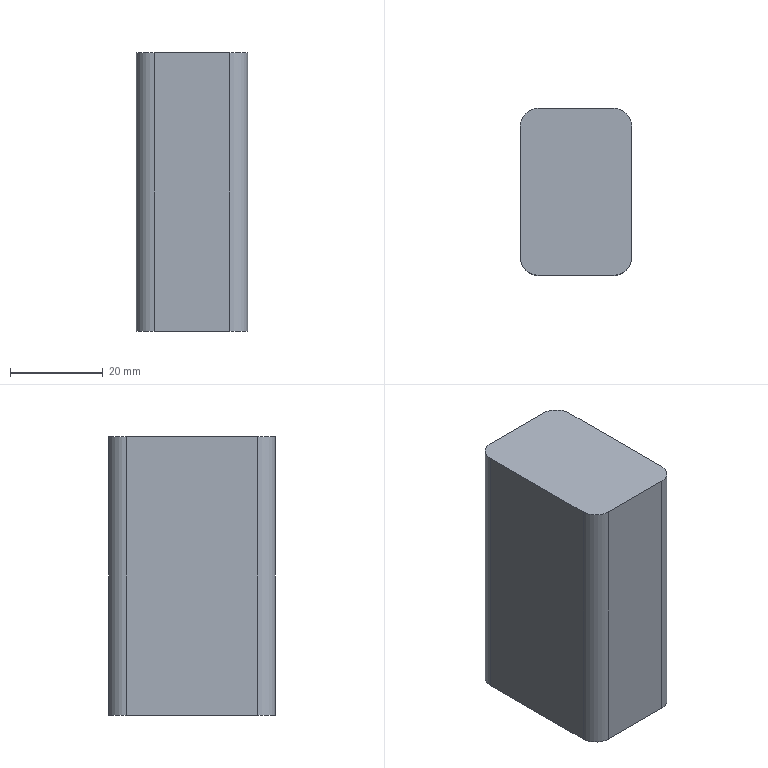Part | NX | 1 solid | 10 faces | box 24 x 36 x 60 mm | volume 51081 mm3 | plane 6 | cylinder 4 | commonest cylinder face diameters 7.68 x4
STEP:
#1=CARTESIAN_POINT('',(244.674,-653.339,1957.099));
#2=VERTEX_POINT('',#1);
#3=CARTESIAN_POINT('',(248.514,-649.499,1957.099));
#4=VERTEX_POINT('',#3);
#5=CARTESIAN_POINT('',(248.514,-653.339,1957.099));
#6=DIRECTION('',(0.,0.,-1.));
#7=DIRECTION('',(-1.,0.,0.));
#8=AXIS2_PLACEMENT_3D('',#5,#6,#7);
#9=CIRCLE('',#8,3.84);
#10=EDGE_CURVE('',#2,#4,#9,.T.);
#11=ORIENTED_EDGE('',*,*,#10,.F.);
#12=CARTESIAN_POINT('',(244.674,-653.339,2017.099));
#13=VERTEX_POINT('',#12);
#14=CARTESIAN_POINT('',(244.674,-653.339,2017.099));
#15=DIRECTION('',(0.,0.,-1.));
#16=VECTOR('',#15,1.);
#17=LINE('',#14,#16);
#18=EDGE_CURVE('',#13,#2,#17,.T.);
#19=ORIENTED_EDGE('',*,*,#18,.F.);
#20=CARTESIAN_POINT('',(248.514,-649.499,2017.099));
#21=VERTEX_POINT('',#20);
#22=CARTESIAN_POINT('',(248.514,-653.339,2017.099));
#23=DIRECTION('',(0.,0.,-1.));
#24=DIRECTION('',(-1.,0.,0.));
#25=AXIS2_PLACEMENT_3D('',#22,#23,#24);
#26=CIRCLE('',#25,3.84);
#27=EDGE_CURVE('',#13,#21,#26,.T.);
#28=ORIENTED_EDGE('',*,*,#27,.T.);
#29=CARTESIAN_POINT('',(248.514,-649.499,2017.099));
#30=DIRECTION('',(0.,0.,-1.));
#31=VECTOR('',#30,1.);
#32=LINE('',#29,#31);
#33=EDGE_CURVE('',#21,#4,#32,.T.);
#34=ORIENTED_EDGE('',*,*,#33,.T.);
#35=EDGE_LOOP('',(#11,#19,#28,#34));
#36=FACE_OUTER_BOUND('',#35,.T.);
#37=CARTESIAN_POINT('',(248.514,-653.339,2017.099));
#38=DIRECTION('',(0.,0.,-1.));
#39=DIRECTION('',(1.,0.,0.));
#40=AXIS2_PLACEMENT_3D('',#37,#38,#39);
#41=CYLINDRICAL_SURFACE('',#40,3.84);
#42=ADVANCED_FACE('',(#36),#41,.T.);
#43=CARTESIAN_POINT('',(264.834,-649.499,1957.099));
#44=VERTEX_POINT('',#43);
#45=CARTESIAN_POINT('',(248.514,-649.499,1957.099));
#46=DIRECTION('',(1.,0.,0.));
#47=VECTOR('',#46,1.);
#48=LINE('',#45,#47);
#49=EDGE_CURVE('',#4,#44,#48,.T.);
#50=ORIENTED_EDGE('',*,*,#49,.F.);
#51=ORIENTED_EDGE('',*,*,#33,.F.);
#52=CARTESIAN_POINT('',(264.834,-649.499,2017.099));
#53=VERTEX_POINT('',#52);
#54=CARTESIAN_POINT('',(248.514,-649.499,2017.099));
#55=DIRECTION('',(1.,0.,0.));
#56=VECTOR('',#55,1.);
#57=LINE('',#54,#56);
#58=EDGE_CURVE('',#21,#53,#57,.T.);
#59=ORIENTED_EDGE('',*,*,#58,.T.);
#60=CARTESIAN_POINT('',(264.834,-649.499,2017.099));
#61=DIRECTION('',(0.,0.,-1.));
#62=VECTOR('',#61,1.);
#63=LINE('',#60,#62);
#64=EDGE_CURVE('',#53,#44,#63,.T.);
#65=ORIENTED_EDGE('',*,*,#64,.T.);
#66=EDGE_LOOP('',(#50,#51,#59,#65));
#67=FACE_OUTER_BOUND('',#66,.T.);
#68=CARTESIAN_POINT('',(248.514,-649.499,2017.099));
#69=DIRECTION('',(0.,-1.,0.));
#70=DIRECTION('',(0.,0.,-1.));
#71=AXIS2_PLACEMENT_3D('',#68,#69,#70);
#72=PLANE('',#71);
#73=ADVANCED_FACE('',(#67),#72,.F.);
#74=CARTESIAN_POINT('',(268.674,-653.339,1957.099));
#75=VERTEX_POINT('',#74);
#76=CARTESIAN_POINT('',(264.834,-653.339,1957.099));
#77=DIRECTION('',(0.,0.,-1.));
#78=DIRECTION('',(-1.,0.,0.));
#79=AXIS2_PLACEMENT_3D('',#76,#77,#78);
#80=CIRCLE('',#79,3.84);
#81=EDGE_CURVE('',#44,#75,#80,.T.);
#82=ORIENTED_EDGE('',*,*,#81,.F.);
#83=ORIENTED_EDGE('',*,*,#64,.F.);
#84=CARTESIAN_POINT('',(268.674,-653.339,2017.099));
#85=VERTEX_POINT('',#84);
#86=CARTESIAN_POINT('',(264.834,-653.339,2017.099));
#87=DIRECTION('',(0.,0.,-1.));
#88=DIRECTION('',(-1.,0.,0.));
#89=AXIS2_PLACEMENT_3D('',#86,#87,#88);
#90=CIRCLE('',#89,3.84);
#91=EDGE_CURVE('',#53,#85,#90,.T.);
#92=ORIENTED_EDGE('',*,*,#91,.T.);
#93=CARTESIAN_POINT('',(268.674,-653.339,2017.099));
#94=DIRECTION('',(0.,0.,-1.));
#95=VECTOR('',#94,1.);
#96=LINE('',#93,#95);
#97=EDGE_CURVE('',#85,#75,#96,.T.);
#98=ORIENTED_EDGE('',*,*,#97,.T.);
#99=EDGE_LOOP('',(#82,#83,#92,#98));
#100=FACE_OUTER_BOUND('',#99,.T.);
#101=CARTESIAN_POINT('',(264.834,-653.339,2017.099));
#102=DIRECTION('',(0.,0.,-1.));
#103=DIRECTION('',(1.,0.,0.));
#104=AXIS2_PLACEMENT_3D('',#101,#102,#103);
#105=CYLINDRICAL_SURFACE('',#104,3.84);
#106=ADVANCED_FACE('',(#100),#105,.T.);
#107=CARTESIAN_POINT('',(268.674,-681.659,1957.099));
#108=VERTEX_POINT('',#107);
#109=CARTESIAN_POINT('',(268.674,-653.339,1957.099));
#110=DIRECTION('',(0.,-1.,0.));
#111=VECTOR('',#110,1.);
#112=LINE('',#109,#111);
#113=EDGE_CURVE('',#75,#108,#112,.T.);
#114=ORIENTED_EDGE('',*,*,#113,.F.);
#115=ORIENTED_EDGE('',*,*,#97,.F.);
#116=CARTESIAN_POINT('',(268.674,-681.659,2017.099));
#117=VERTEX_POINT('',#116);
#118=CARTESIAN_POINT('',(268.674,-653.339,2017.099));
#119=DIRECTION('',(0.,-1.,0.));
#120=VECTOR('',#119,1.);
#121=LINE('',#118,#120);
#122=EDGE_CURVE('',#85,#117,#121,.T.);
#123=ORIENTED_EDGE('',*,*,#122,.T.);
#124=CARTESIAN_POINT('',(268.674,-681.659,2017.099));
#125=DIRECTION('',(0.,0.,-1.));
#126=VECTOR('',#125,1.);
#127=LINE('',#124,#126);
#128=EDGE_CURVE('',#117,#108,#127,.T.);
#129=ORIENTED_EDGE('',*,*,#128,.T.);
#130=EDGE_LOOP('',(#114,#115,#123,#129));
#131=FACE_OUTER_BOUND('',#130,.T.);
#132=CARTESIAN_POINT('',(268.674,-653.339,2017.099));
#133=DIRECTION('',(-1.,0.,0.));
#134=DIRECTION('',(0.,1.,0.));
#135=AXIS2_PLACEMENT_3D('',#132,#133,#134);
#136=PLANE('',#135);
#137=ADVANCED_FACE('',(#131),#136,.F.);
#138=CARTESIAN_POINT('',(264.834,-685.499,1957.099));
#139=VERTEX_POINT('',#138);
#140=CARTESIAN_POINT('',(264.834,-681.659,1957.099));
#141=DIRECTION('',(0.,0.,-1.));
#142=DIRECTION('',(-1.,0.,0.));
#143=AXIS2_PLACEMENT_3D('',#140,#141,#142);
#144=CIRCLE('',#143,3.84);
#145=EDGE_CURVE('',#108,#139,#144,.T.);
#146=ORIENTED_EDGE('',*,*,#145,.F.);
#147=ORIENTED_EDGE('',*,*,#128,.F.);
#148=CARTESIAN_POINT('',(264.834,-685.499,2017.099));
#149=VERTEX_POINT('',#148);
#150=CARTESIAN_POINT('',(264.834,-681.659,2017.099));
#151=DIRECTION('',(0.,0.,-1.));
#152=DIRECTION('',(-1.,0.,0.));
#153=AXIS2_PLACEMENT_3D('',#150,#151,#152);
#154=CIRCLE('',#153,3.84);
#155=EDGE_CURVE('',#117,#149,#154,.T.);
#156=ORIENTED_EDGE('',*,*,#155,.T.);
#157=CARTESIAN_POINT('',(264.834,-685.499,2017.099));
#158=DIRECTION('',(0.,0.,-1.));
#159=VECTOR('',#158,1.);
#160=LINE('',#157,#159);
#161=EDGE_CURVE('',#149,#139,#160,.T.);
#162=ORIENTED_EDGE('',*,*,#161,.T.);
#163=EDGE_LOOP('',(#146,#147,#156,#162));
#164=FACE_OUTER_BOUND('',#163,.T.);
#165=CARTESIAN_POINT('',(264.834,-681.659,2017.099));
#166=DIRECTION('',(0.,0.,-1.));
#167=DIRECTION('',(1.,0.,0.));
#168=AXIS2_PLACEMENT_3D('',#165,#166,#167);
#169=CYLINDRICAL_SURFACE('',#168,3.84);
#170=ADVANCED_FACE('',(#164),#169,.T.);
#171=CARTESIAN_POINT('',(248.514,-685.499,1957.099));
#172=VERTEX_POINT('',#171);
#173=CARTESIAN_POINT('',(264.834,-685.499,1957.099));
#174=DIRECTION('',(-1.,0.,0.));
#175=VECTOR('',#174,1.);
#176=LINE('',#173,#175);
#177=EDGE_CURVE('',#139,#172,#176,.T.);
#178=ORIENTED_EDGE('',*,*,#177,.F.);
#179=ORIENTED_EDGE('',*,*,#161,.F.);
#180=CARTESIAN_POINT('',(248.514,-685.499,2017.099));
#181=VERTEX_POINT('',#180);
#182=CARTESIAN_POINT('',(264.834,-685.499,2017.099));
#183=DIRECTION('',(-1.,0.,0.));
#184=VECTOR('',#183,1.);
#185=LINE('',#182,#184);
#186=EDGE_CURVE('',#149,#181,#185,.T.);
#187=ORIENTED_EDGE('',*,*,#186,.T.);
#188=CARTESIAN_POINT('',(248.514,-685.499,2017.099));
#189=DIRECTION('',(0.,0.,-1.));
#190=VECTOR('',#189,1.);
#191=LINE('',#188,#190);
#192=EDGE_CURVE('',#181,#172,#191,.T.);
#193=ORIENTED_EDGE('',*,*,#192,.T.);
#194=EDGE_LOOP('',(#178,#179,#187,#193));
#195=FACE_OUTER_BOUND('',#194,.T.);
#196=CARTESIAN_POINT('',(264.834,-685.499,2017.099));
#197=DIRECTION('',(0.,1.,0.));
#198=DIRECTION('',(1.,0.,0.));
#199=AXIS2_PLACEMENT_3D('',#196,#197,#198);
#200=PLANE('',#199);
#201=ADVANCED_FACE('',(#195),#200,.F.);
#202=CARTESIAN_POINT('',(244.674,-681.659,1957.099));
#203=VERTEX_POINT('',#202);
#204=CARTESIAN_POINT('',(248.514,-681.659,1957.099));
#205=DIRECTION('',(0.,0.,-1.));
#206=DIRECTION('',(-1.,0.,0.));
#207=AXIS2_PLACEMENT_3D('',#204,#205,#206);
#208=CIRCLE('',#207,3.84);
#209=EDGE_CURVE('',#172,#203,#208,.T.);
#210=ORIENTED_EDGE('',*,*,#209,.F.);
#211=ORIENTED_EDGE('',*,*,#192,.F.);
#212=CARTESIAN_POINT('',(244.674,-681.659,2017.099));
#213=VERTEX_POINT('',#212);
#214=CARTESIAN_POINT('',(248.514,-681.659,2017.099));
#215=DIRECTION('',(0.,0.,-1.));
#216=DIRECTION('',(-1.,0.,0.));
#217=AXIS2_PLACEMENT_3D('',#214,#215,#216);
#218=CIRCLE('',#217,3.84);
#219=EDGE_CURVE('',#181,#213,#218,.T.);
#220=ORIENTED_EDGE('',*,*,#219,.T.);
#221=CARTESIAN_POINT('',(244.674,-681.659,2017.099));
#222=DIRECTION('',(0.,0.,-1.));
#223=VECTOR('',#222,1.);
#224=LINE('',#221,#223);
#225=EDGE_CURVE('',#213,#203,#224,.T.);
#226=ORIENTED_EDGE('',*,*,#225,.T.);
#227=EDGE_LOOP('',(#210,#211,#220,#226));
#228=FACE_OUTER_BOUND('',#227,.T.);
#229=CARTESIAN_POINT('',(248.514,-681.659,2017.099));
#230=DIRECTION('',(0.,0.,-1.));
#231=DIRECTION('',(1.,0.,0.));
#232=AXIS2_PLACEMENT_3D('',#229,#230,#231);
#233=CYLINDRICAL_SURFACE('',#232,3.84);
#234=ADVANCED_FACE('',(#228),#233,.T.);
#235=CARTESIAN_POINT('',(244.674,-681.659,1957.099));
#236=DIRECTION('',(0.,1.,0.));
#237=VECTOR('',#236,1.);
#238=LINE('',#235,#237);
#239=EDGE_CURVE('',#203,#2,#238,.T.);
#240=ORIENTED_EDGE('',*,*,#239,.F.);
#241=ORIENTED_EDGE('',*,*,#225,.F.);
#242=CARTESIAN_POINT('',(244.674,-681.659,2017.099));
#243=DIRECTION('',(0.,1.,0.));
#244=VECTOR('',#243,1.);
#245=LINE('',#242,#244);
#246=EDGE_CURVE('',#213,#13,#245,.T.);
#247=ORIENTED_EDGE('',*,*,#246,.T.);
#248=ORIENTED_EDGE('',*,*,#18,.T.);
#249=EDGE_LOOP('',(#240,#241,#247,#248));
#250=FACE_OUTER_BOUND('',#249,.T.);
#251=CARTESIAN_POINT('',(244.674,-681.659,2017.099));
#252=DIRECTION('',(1.,0.,0.));
#253=DIRECTION('',(0.,-1.,0.));
#254=AXIS2_PLACEMENT_3D('',#251,#252,#253);
#255=PLANE('',#254);
#256=ADVANCED_FACE('',(#250),#255,.F.);
#257=ORIENTED_EDGE('',*,*,#27,.F.);
#258=ORIENTED_EDGE('',*,*,#246,.F.);
#259=ORIENTED_EDGE('',*,*,#219,.F.);
#260=ORIENTED_EDGE('',*,*,#186,.F.);
#261=ORIENTED_EDGE('',*,*,#155,.F.);
#262=ORIENTED_EDGE('',*,*,#122,.F.);
#263=ORIENTED_EDGE('',*,*,#91,.F.);
#264=ORIENTED_EDGE('',*,*,#58,.F.);
#265=EDGE_LOOP('',(#257,#258,#259,#260,#261,#262,#263,#264));
#266=FACE_OUTER_BOUND('',#265,.T.);
#267=CARTESIAN_POINT('',(248.514,-653.339,2017.099));
#268=DIRECTION('',(0.,0.,1.));
#269=DIRECTION('',(-1.,0.,0.));
#270=AXIS2_PLACEMENT_3D('',#267,#268,#269);
#271=PLANE('',#270);
#272=ADVANCED_FACE('',(#266),#271,.T.);
#273=ORIENTED_EDGE('',*,*,#10,.T.);
#274=ORIENTED_EDGE('',*,*,#49,.T.);
#275=ORIENTED_EDGE('',*,*,#81,.T.);
#276=ORIENTED_EDGE('',*,*,#113,.T.);
#277=ORIENTED_EDGE('',*,*,#145,.T.);
#278=ORIENTED_EDGE('',*,*,#177,.T.);
#279=ORIENTED_EDGE('',*,*,#209,.T.);
#280=ORIENTED_EDGE('',*,*,#239,.T.);
#281=EDGE_LOOP('',(#273,#274,#275,#276,#277,#278,#279,#280));
#282=FACE_OUTER_BOUND('',#281,.T.);
#283=CARTESIAN_POINT('',(248.514,-653.339,1957.099));
#284=DIRECTION('',(0.,0.,1.));
#285=DIRECTION('',(-1.,0.,0.));
#286=AXIS2_PLACEMENT_3D('',#283,#284,#285);
#287=PLANE('',#286);
#288=ADVANCED_FACE('',(#282),#287,.F.);
#289=CLOSED_SHELL('',(#42,#73,#106,#137,#170,#201,#234,#256,#272,#288));
#290=MANIFOLD_SOLID_BREP('',#289);
#291=(LENGTH_UNIT()NAMED_UNIT(*)SI_UNIT(.MILLI.,.METRE.));
#292=UNCERTAINTY_MEASURE_WITH_UNIT(LENGTH_MEASURE(0.00002),#291,'','');
#293=(NAMED_UNIT(*)PLANE_ANGLE_UNIT()SI_UNIT($,.RADIAN.));
#294=PLANE_ANGLE_MEASURE_WITH_UNIT(PLANE_ANGLE_MEASURE(0.01745),#293);
#295=DIMENSIONAL_EXPONENTS(0.,0.,0.,0.,0.,0.,0.);
#296=(CONVERSION_BASED_UNIT('DEGREE',#294)NAMED_UNIT(#295)PLANE_ANGLE_UNIT());
#297=(NAMED_UNIT(*)SI_UNIT($,.STERADIAN.)SOLID_ANGLE_UNIT());
#298=(GEOMETRIC_REPRESENTATION_CONTEXT(3)GLOBAL_UNCERTAINTY_ASSIGNED_CONTEXT((#292))GLOBAL_UNIT_ASSIGNED_CONTEXT((#291,#296,#297))REPRESENTATION_CONTEXT('',''));
#299=ADVANCED_BREP_SHAPE_REPRESENTATION('',(#290),#298);